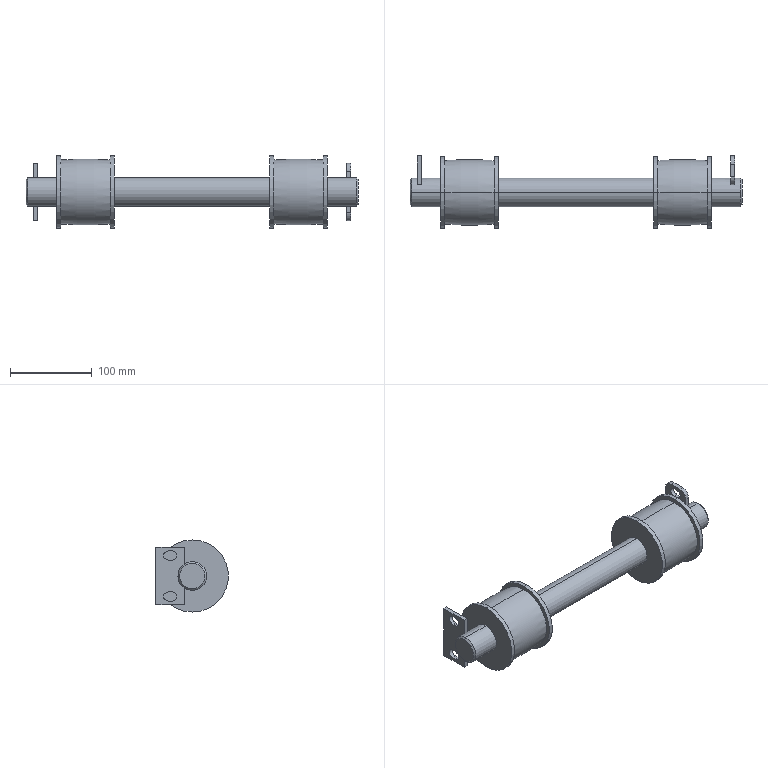Part | SolidWorks | features ICE 3, Fillet 1, Revolution 1 | 3 solids | 70 faces | box 405 x 88.5 x 88 mm | volume 988805 mm3 | plane 36 | cylinder 26 | torus 4 | cone 4 | commonest cylinder face diameters 11 x8 88 x8 35 x6 20 x4